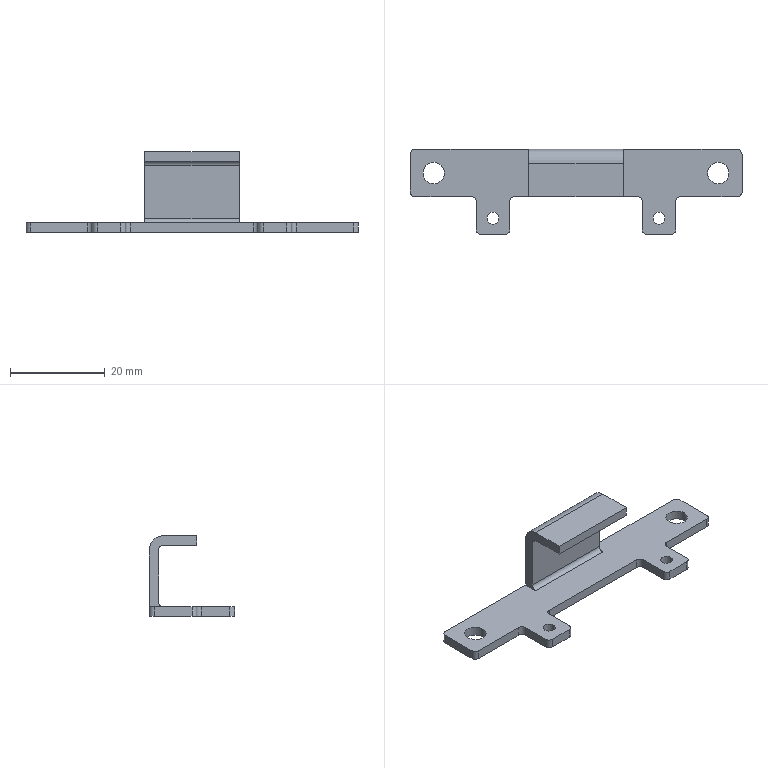Part | SolidWorks | features Fillet 4, ICE 4, 3DProfileFeature 1, Extrusion 1, HoleWzd 1 | 1 solid | 43 faces | box 70 x 18 x 17 mm | volume 2429 mm3 | cylinder 23 | plane 20 | commonest cylinder face diameters 2 x14 2.5 x4 4.5 x4 6 x1
STEP:
#1=CARTESIAN_POINT('',(-18.75,-9.5,0.));
#2=VERTEX_POINT('',#1);
#3=CARTESIAN_POINT('',(-16.25,-9.5,0.));
#4=VERTEX_POINT('',#3);
#5=CARTESIAN_POINT('',(-17.5,-9.5,0.));
#6=DIRECTION('',(0.,0.,1.));
#7=DIRECTION('',(1.,0.,0.));
#8=AXIS2_PLACEMENT_3D('',#5,#6,#7);
#9=CIRCLE('',#8,1.25);
#10=EDGE_CURVE('',#2,#4,#9,.T.);
#11=ORIENTED_EDGE('',*,*,#10,.F.);
#12=CARTESIAN_POINT('',(-18.75,-9.5,2.));
#13=VERTEX_POINT('',#12);
#14=CARTESIAN_POINT('',(-18.75,-9.5,2.));
#15=DIRECTION('',(0.,0.,1.));
#16=VECTOR('',#15,1000.);
#17=LINE('',#14,#16);
#18=EDGE_CURVE('',#2,#13,#17,.T.);
#19=ORIENTED_EDGE('',*,*,#18,.T.);
#20=CARTESIAN_POINT('',(-16.25,-9.5,2.));
#21=VERTEX_POINT('',#20);
#22=CARTESIAN_POINT('',(-17.5,-9.5,2.));
#23=DIRECTION('',(0.,0.,1.));
#24=DIRECTION('',(1.,0.,0.));
#25=AXIS2_PLACEMENT_3D('',#22,#23,#24);
#26=CIRCLE('',#25,1.25);
#27=EDGE_CURVE('',#13,#21,#26,.T.);
#28=ORIENTED_EDGE('',*,*,#27,.T.);
#29=CARTESIAN_POINT('',(-16.25,-9.5,2.));
#30=DIRECTION('',(0.,0.,1.));
#31=VECTOR('',#30,1000.);
#32=LINE('',#29,#31);
#33=EDGE_CURVE('',#4,#21,#32,.T.);
#34=ORIENTED_EDGE('',*,*,#33,.F.);
#35=EDGE_LOOP('',(#11,#19,#28,#34));
#36=FACE_OUTER_BOUND('',#35,.T.);
#37=CARTESIAN_POINT('',(-17.5,-9.5,2.));
#38=DIRECTION('',(0.,0.,1.));
#39=DIRECTION('',(1.,0.,0.));
#40=AXIS2_PLACEMENT_3D('',#37,#38,#39);
#41=CYLINDRICAL_SURFACE('',#40,1.25);
#42=ADVANCED_FACE('',(#36),#41,.F.);
#43=CARTESIAN_POINT('',(16.25,-9.5,0.));
#44=VERTEX_POINT('',#43);
#45=CARTESIAN_POINT('',(18.75,-9.5,0.));
#46=VERTEX_POINT('',#45);
#47=CARTESIAN_POINT('',(17.5,-9.5,0.));
#48=DIRECTION('',(0.,0.,1.));
#49=DIRECTION('',(1.,0.,0.));
#50=AXIS2_PLACEMENT_3D('',#47,#48,#49);
#51=CIRCLE('',#50,1.25);
#52=EDGE_CURVE('',#44,#46,#51,.T.);
#53=ORIENTED_EDGE('',*,*,#52,.F.);
#54=CARTESIAN_POINT('',(16.25,-9.5,2.));
#55=VERTEX_POINT('',#54);
#56=CARTESIAN_POINT('',(16.25,-9.5,2.));
#57=DIRECTION('',(0.,0.,1.));
#58=VECTOR('',#57,1000.);
#59=LINE('',#56,#58);
#60=EDGE_CURVE('',#44,#55,#59,.T.);
#61=ORIENTED_EDGE('',*,*,#60,.T.);
#62=CARTESIAN_POINT('',(18.75,-9.5,2.));
#63=VERTEX_POINT('',#62);
#64=CARTESIAN_POINT('',(17.5,-9.5,2.));
#65=DIRECTION('',(0.,0.,1.));
#66=DIRECTION('',(1.,0.,0.));
#67=AXIS2_PLACEMENT_3D('',#64,#65,#66);
#68=CIRCLE('',#67,1.25);
#69=EDGE_CURVE('',#55,#63,#68,.T.);
#70=ORIENTED_EDGE('',*,*,#69,.T.);
#71=CARTESIAN_POINT('',(18.75,-9.5,2.));
#72=DIRECTION('',(0.,0.,1.));
#73=VECTOR('',#72,1000.);
#74=LINE('',#71,#73);
#75=EDGE_CURVE('',#46,#63,#74,.T.);
#76=ORIENTED_EDGE('',*,*,#75,.F.);
#77=EDGE_LOOP('',(#53,#61,#70,#76));
#78=FACE_OUTER_BOUND('',#77,.T.);
#79=CARTESIAN_POINT('',(17.5,-9.5,2.));
#80=DIRECTION('',(0.,0.,1.));
#81=DIRECTION('',(1.,0.,0.));
#82=AXIS2_PLACEMENT_3D('',#79,#80,#81);
#83=CYLINDRICAL_SURFACE('',#82,1.25);
#84=ADVANCED_FACE('',(#78),#83,.F.);
#85=CARTESIAN_POINT('',(-32.25,0.,0.));
#86=VERTEX_POINT('',#85);
#87=CARTESIAN_POINT('',(-27.75,0.,0.));
#88=VERTEX_POINT('',#87);
#89=CARTESIAN_POINT('',(-30.,0.,0.));
#90=DIRECTION('',(0.,0.,1.));
#91=DIRECTION('',(1.,0.,0.));
#92=AXIS2_PLACEMENT_3D('',#89,#90,#91);
#93=CIRCLE('',#92,2.25);
#94=EDGE_CURVE('',#86,#88,#93,.T.);
#95=ORIENTED_EDGE('',*,*,#94,.F.);
#96=CARTESIAN_POINT('',(-32.25,0.,2.));
#97=VERTEX_POINT('',#96);
#98=CARTESIAN_POINT('',(-32.25,0.,-6.));
#99=DIRECTION('',(0.,0.,1.));
#100=VECTOR('',#99,1000.);
#101=LINE('',#98,#100);
#102=EDGE_CURVE('',#86,#97,#101,.T.);
#103=ORIENTED_EDGE('',*,*,#102,.T.);
#104=CARTESIAN_POINT('',(-27.75,0.,2.));
#105=VERTEX_POINT('',#104);
#106=CARTESIAN_POINT('',(-30.,0.,2.));
#107=DIRECTION('',(0.,0.,1.));
#108=DIRECTION('',(1.,0.,0.));
#109=AXIS2_PLACEMENT_3D('',#106,#107,#108);
#110=CIRCLE('',#109,2.25);
#111=EDGE_CURVE('',#97,#105,#110,.T.);
#112=ORIENTED_EDGE('',*,*,#111,.T.);
#113=CARTESIAN_POINT('',(-27.75,0.,-6.));
#114=DIRECTION('',(0.,0.,1.));
#115=VECTOR('',#114,1000.);
#116=LINE('',#113,#115);
#117=EDGE_CURVE('',#88,#105,#116,.T.);
#118=ORIENTED_EDGE('',*,*,#117,.F.);
#119=EDGE_LOOP('',(#95,#103,#112,#118));
#120=FACE_OUTER_BOUND('',#119,.T.);
#121=CARTESIAN_POINT('',(-30.,0.,-6.));
#122=DIRECTION('',(0.,0.,1.));
#123=DIRECTION('',(1.,0.,0.));
#124=AXIS2_PLACEMENT_3D('',#121,#122,#123);
#125=CYLINDRICAL_SURFACE('',#124,2.25);
#126=ADVANCED_FACE('',(#120),#125,.F.);
#127=CARTESIAN_POINT('',(27.75,0.,0.));
#128=VERTEX_POINT('',#127);
#129=CARTESIAN_POINT('',(32.25,0.,0.));
#130=VERTEX_POINT('',#129);
#131=CARTESIAN_POINT('',(30.,0.,0.));
#132=DIRECTION('',(0.,0.,1.));
#133=DIRECTION('',(1.,0.,0.));
#134=AXIS2_PLACEMENT_3D('',#131,#132,#133);
#135=CIRCLE('',#134,2.25);
#136=EDGE_CURVE('',#128,#130,#135,.T.);
#137=ORIENTED_EDGE('',*,*,#136,.F.);
#138=CARTESIAN_POINT('',(27.75,0.,2.));
#139=VERTEX_POINT('',#138);
#140=CARTESIAN_POINT('',(27.75,0.,-6.));
#141=DIRECTION('',(0.,0.,1.));
#142=VECTOR('',#141,1000.);
#143=LINE('',#140,#142);
#144=EDGE_CURVE('',#128,#139,#143,.T.);
#145=ORIENTED_EDGE('',*,*,#144,.T.);
#146=CARTESIAN_POINT('',(32.25,0.,2.));
#147=VERTEX_POINT('',#146);
#148=CARTESIAN_POINT('',(30.,0.,2.));
#149=DIRECTION('',(0.,0.,1.));
#150=DIRECTION('',(1.,0.,0.));
#151=AXIS2_PLACEMENT_3D('',#148,#149,#150);
#152=CIRCLE('',#151,2.25);
#153=EDGE_CURVE('',#139,#147,#152,.T.);
#154=ORIENTED_EDGE('',*,*,#153,.T.);
#155=CARTESIAN_POINT('',(32.25,0.,-6.));
#156=DIRECTION('',(0.,0.,1.));
#157=VECTOR('',#156,1000.);
#158=LINE('',#155,#157);
#159=EDGE_CURVE('',#130,#147,#158,.T.);
#160=ORIENTED_EDGE('',*,*,#159,.F.);
#161=EDGE_LOOP('',(#137,#145,#154,#160));
#162=FACE_OUTER_BOUND('',#161,.T.);
#163=CARTESIAN_POINT('',(30.,0.,-6.));
#164=DIRECTION('',(0.,0.,1.));
#165=DIRECTION('',(1.,0.,0.));
#166=AXIS2_PLACEMENT_3D('',#163,#164,#165);
#167=CYLINDRICAL_SURFACE('',#166,2.25);
#168=ADVANCED_FACE('',(#162),#167,.F.);
#169=CARTESIAN_POINT('',(-13.,-5.,2.));
#170=VERTEX_POINT('',#169);
#171=CARTESIAN_POINT('',(13.,-5.,2.));
#172=VERTEX_POINT('',#171);
#173=CARTESIAN_POINT('',(-35.,-5.,2.));
#174=DIRECTION('',(1.,0.,0.));
#175=VECTOR('',#174,1000.);
#176=LINE('',#173,#175);
#177=EDGE_CURVE('',#170,#172,#176,.T.);
#178=ORIENTED_EDGE('',*,*,#177,.F.);
#179=CARTESIAN_POINT('',(-13.,-5.,0.));
#180=VERTEX_POINT('',#179);
#181=CARTESIAN_POINT('',(-13.,-5.,0.));
#182=DIRECTION('',(0.,0.,-1.));
#183=VECTOR('',#182,1000.);
#184=LINE('',#181,#183);
#185=EDGE_CURVE('',#170,#180,#184,.T.);
#186=ORIENTED_EDGE('',*,*,#185,.T.);
#187=CARTESIAN_POINT('',(13.,-5.,0.));
#188=VERTEX_POINT('',#187);
#189=CARTESIAN_POINT('',(-35.,-5.,0.));
#190=DIRECTION('',(1.,0.,0.));
#191=VECTOR('',#190,1000.);
#192=LINE('',#189,#191);
#193=EDGE_CURVE('',#180,#188,#192,.T.);
#194=ORIENTED_EDGE('',*,*,#193,.T.);
#195=CARTESIAN_POINT('',(13.,-5.,2.));
#196=DIRECTION('',(0.,0.,1.));
#197=VECTOR('',#196,1000.);
#198=LINE('',#195,#197);
#199=EDGE_CURVE('',#188,#172,#198,.T.);
#200=ORIENTED_EDGE('',*,*,#199,.T.);
#201=EDGE_LOOP('',(#178,#186,#194,#200));
#202=FACE_OUTER_BOUND('',#201,.T.);
#203=CARTESIAN_POINT('',(-35.,-5.,2.));
#204=DIRECTION('',(0.,1.,0.));
#205=DIRECTION('',(0.,0.,1.));
#206=AXIS2_PLACEMENT_3D('',#203,#204,#205);
#207=PLANE('',#206);
#208=ADVANCED_FACE('',(#202),#207,.F.);
#209=CARTESIAN_POINT('',(22.,-5.,2.));
#210=VERTEX_POINT('',#209);
#211=CARTESIAN_POINT('',(34.,-5.,2.));
#212=VERTEX_POINT('',#211);
#213=CARTESIAN_POINT('',(-35.,-5.,2.));
#214=DIRECTION('',(1.,0.,0.));
#215=VECTOR('',#214,1000.);
#216=LINE('',#213,#215);
#217=EDGE_CURVE('',#210,#212,#216,.T.);
#218=ORIENTED_EDGE('',*,*,#217,.F.);
#219=CARTESIAN_POINT('',(22.,-5.,0.));
#220=VERTEX_POINT('',#219);
#221=CARTESIAN_POINT('',(22.,-5.,0.));
#222=DIRECTION('',(0.,0.,-1.));
#223=VECTOR('',#222,1000.);
#224=LINE('',#221,#223);
#225=EDGE_CURVE('',#210,#220,#224,.T.);
#226=ORIENTED_EDGE('',*,*,#225,.T.);
#227=CARTESIAN_POINT('',(34.,-5.,0.));
#228=VERTEX_POINT('',#227);
#229=CARTESIAN_POINT('',(-35.,-5.,0.));
#230=DIRECTION('',(1.,0.,0.));
#231=VECTOR('',#230,1000.);
#232=LINE('',#229,#231);
#233=EDGE_CURVE('',#220,#228,#232,.T.);
#234=ORIENTED_EDGE('',*,*,#233,.T.);
#235=CARTESIAN_POINT('',(34.,-5.,2.));
#236=DIRECTION('',(0.,0.,1.));
#237=VECTOR('',#236,1000.);
#238=LINE('',#235,#237);
#239=EDGE_CURVE('',#228,#212,#238,.T.);
#240=ORIENTED_EDGE('',*,*,#239,.T.);
#241=EDGE_LOOP('',(#218,#226,#234,#240));
#242=FACE_OUTER_BOUND('',#241,.T.);
#243=CARTESIAN_POINT('',(-35.,-5.,2.));
#244=DIRECTION('',(0.,1.,0.));
#245=DIRECTION('',(0.,0.,1.));
#246=AXIS2_PLACEMENT_3D('',#243,#244,#245);
#247=PLANE('',#246);
#248=ADVANCED_FACE('',(#242),#247,.F.);
#249=CARTESIAN_POINT('',(-34.,-5.,0.));
#250=VERTEX_POINT('',#249);
#251=CARTESIAN_POINT('',(-22.,-5.,0.));
#252=VERTEX_POINT('',#251);
#253=CARTESIAN_POINT('',(-35.,-5.,0.));
#254=DIRECTION('',(1.,0.,0.));
#255=VECTOR('',#254,1000.);
#256=LINE('',#253,#255);
#257=EDGE_CURVE('',#250,#252,#256,.T.);
#258=ORIENTED_EDGE('',*,*,#257,.T.);
#259=CARTESIAN_POINT('',(-22.,-5.,2.));
#260=VERTEX_POINT('',#259);
#261=CARTESIAN_POINT('',(-22.,-5.,2.));
#262=DIRECTION('',(0.,0.,1.));
#263=VECTOR('',#262,1000.);
#264=LINE('',#261,#263);
#265=EDGE_CURVE('',#252,#260,#264,.T.);
#266=ORIENTED_EDGE('',*,*,#265,.T.);
#267=CARTESIAN_POINT('',(-34.,-5.,2.));
#268=VERTEX_POINT('',#267);
#269=CARTESIAN_POINT('',(-35.,-5.,2.));
#270=DIRECTION('',(1.,0.,0.));
#271=VECTOR('',#270,1000.);
#272=LINE('',#269,#271);
#273=EDGE_CURVE('',#268,#260,#272,.T.);
#274=ORIENTED_EDGE('',*,*,#273,.F.);
#275=CARTESIAN_POINT('',(-34.,-5.,2.));
#276=DIRECTION('',(0.,0.,-1.));
#277=VECTOR('',#276,1000.);
#278=LINE('',#275,#277);
#279=EDGE_CURVE('',#268,#250,#278,.T.);
#280=ORIENTED_EDGE('',*,*,#279,.T.);
#281=EDGE_LOOP('',(#258,#266,#274,#280));
#282=FACE_OUTER_BOUND('',#281,.T.);
#283=CARTESIAN_POINT('',(-35.,-5.,2.));
#284=DIRECTION('',(0.,1.,0.));
#285=DIRECTION('',(0.,0.,1.));
#286=AXIS2_PLACEMENT_3D('',#283,#284,#285);
#287=PLANE('',#286);
#288=ADVANCED_FACE('',(#282),#287,.F.);
#289=CARTESIAN_POINT('',(-10.,3.,14.));
#290=VERTEX_POINT('',#289);
#291=CARTESIAN_POINT('',(-10.,3.,3.));
#292=VERTEX_POINT('',#291);
#293=CARTESIAN_POINT('',(-10.,3.,17.));
#294=DIRECTION('',(0.,0.,-1.));
#295=VECTOR('',#294,1000.);
#296=LINE('',#293,#295);
#297=EDGE_CURVE('',#290,#292,#296,.T.);
#298=ORIENTED_EDGE('',*,*,#297,.T.);
#299=CARTESIAN_POINT('',(10.,3.,3.));
#300=VERTEX_POINT('',#299);
#301=CARTESIAN_POINT('',(-10.,3.,3.));
#302=DIRECTION('',(1.,0.,0.));
#303=VECTOR('',#302,1000.);
#304=LINE('',#301,#303);
#305=EDGE_CURVE('',#292,#300,#304,.T.);
#306=ORIENTED_EDGE('',*,*,#305,.T.);
#307=CARTESIAN_POINT('',(10.,3.,14.));
#308=VERTEX_POINT('',#307);
#309=CARTESIAN_POINT('',(10.,3.,17.));
#310=DIRECTION('',(0.,0.,-1.));
#311=VECTOR('',#310,1000.);
#312=LINE('',#309,#311);
#313=EDGE_CURVE('',#308,#300,#312,.T.);
#314=ORIENTED_EDGE('',*,*,#313,.F.);
#315=CARTESIAN_POINT('',(-10.,3.,14.));
#316=DIRECTION('',(-1.,0.,0.));
#317=VECTOR('',#316,1000.);
#318=LINE('',#315,#317);
#319=EDGE_CURVE('',#308,#290,#318,.T.);
#320=ORIENTED_EDGE('',*,*,#319,.T.);
#321=EDGE_LOOP('',(#298,#306,#314,#320));
#322=FACE_OUTER_BOUND('',#321,.T.);
#323=CARTESIAN_POINT('',(-10.,3.,17.));
#324=DIRECTION('',(0.,1.,0.));
#325=DIRECTION('',(0.,0.,1.));
#326=AXIS2_PLACEMENT_3D('',#323,#324,#325);
#327=PLANE('',#326);
#328=ADVANCED_FACE('',(#322),#327,.F.);
#329=CARTESIAN_POINT('',(35.,-4.,0.));
#330=VERTEX_POINT('',#329);
#331=CARTESIAN_POINT('',(35.,4.,0.));
#332=VERTEX_POINT('',#331);
#333=CARTESIAN_POINT('',(35.,5.,0.));
#334=DIRECTION('',(0.,1.,0.));
#335=VECTOR('',#334,1000.);
#336=LINE('',#333,#335);
#337=EDGE_CURVE('',#330,#332,#336,.T.);
#338=ORIENTED_EDGE('',*,*,#337,.T.);
#339=CARTESIAN_POINT('',(35.,4.,2.));
#340=VERTEX_POINT('',#339);
#341=CARTESIAN_POINT('',(35.,4.,2.));
#342=DIRECTION('',(0.,0.,1.));
#343=VECTOR('',#342,1000.);
#344=LINE('',#341,#343);
#345=EDGE_CURVE('',#332,#340,#344,.T.);
#346=ORIENTED_EDGE('',*,*,#345,.T.);
#347=CARTESIAN_POINT('',(35.,-4.,2.));
#348=VERTEX_POINT('',#347);
#349=CARTESIAN_POINT('',(35.,5.,2.));
#350=DIRECTION('',(0.,1.,0.));
#351=VECTOR('',#350,1000.);
#352=LINE('',#349,#351);
#353=EDGE_CURVE('',#348,#340,#352,.T.);
#354=ORIENTED_EDGE('',*,*,#353,.F.);
#355=CARTESIAN_POINT('',(35.,-4.,2.));
#356=DIRECTION('',(0.,0.,-1.));
#357=VECTOR('',#356,1000.);
#358=LINE('',#355,#357);
#359=EDGE_CURVE('',#348,#330,#358,.T.);
#360=ORIENTED_EDGE('',*,*,#359,.T.);
#361=EDGE_LOOP('',(#338,#346,#354,#360));
#362=FACE_OUTER_BOUND('',#361,.T.);
#363=CARTESIAN_POINT('',(35.,5.,2.));
#364=DIRECTION('',(-1.,0.,0.));
#365=DIRECTION('',(0.,0.,1.));
#366=AXIS2_PLACEMENT_3D('',#363,#364,#365);
#367=PLANE('',#366);
#368=ADVANCED_FACE('',(#362),#367,.F.);
#369=CARTESIAN_POINT('',(34.,5.,2.));
#370=VERTEX_POINT('',#369);
#371=CARTESIAN_POINT('',(10.,5.,2.));
#372=VERTEX_POINT('',#371);
#373=CARTESIAN_POINT('',(-35.,5.,2.));
#374=DIRECTION('',(-1.,0.,0.));
#375=VECTOR('',#374,1000.);
#376=LINE('',#373,#375);
#377=EDGE_CURVE('',#370,#372,#376,.T.);
#378=ORIENTED_EDGE('',*,*,#377,.F.);
#379=CARTESIAN_POINT('',(34.,5.,0.));
#380=VERTEX_POINT('',#379);
#381=CARTESIAN_POINT('',(34.,5.,2.));
#382=DIRECTION('',(0.,0.,-1.));
#383=VECTOR('',#382,1000.);
#384=LINE('',#381,#383);
#385=EDGE_CURVE('',#370,#380,#384,.T.);
#386=ORIENTED_EDGE('',*,*,#385,.T.);
#387=CARTESIAN_POINT('',(-34.,5.,0.));
#388=VERTEX_POINT('',#387);
#389=CARTESIAN_POINT('',(-35.,5.,0.));
#390=DIRECTION('',(-1.,0.,0.));
#391=VECTOR('',#390,1000.);
#392=LINE('',#389,#391);
#393=EDGE_CURVE('',#380,#388,#392,.T.);
#394=ORIENTED_EDGE('',*,*,#393,.T.);
#395=CARTESIAN_POINT('',(-34.,5.,2.));
#396=VERTEX_POINT('',#395);
#397=CARTESIAN_POINT('',(-34.,5.,2.));
#398=DIRECTION('',(0.,0.,1.));
#399=VECTOR('',#398,1000.);
#400=LINE('',#397,#399);
#401=EDGE_CURVE('',#388,#396,#400,.T.);
#402=ORIENTED_EDGE('',*,*,#401,.T.);
#403=CARTESIAN_POINT('',(-10.,5.,2.));
#404=VERTEX_POINT('',#403);
#405=CARTESIAN_POINT('',(-35.,5.,2.));
#406=DIRECTION('',(-1.,0.,0.));
#407=VECTOR('',#406,1000.);
#408=LINE('',#405,#407);
#409=EDGE_CURVE('',#404,#396,#408,.T.);
#410=ORIENTED_EDGE('',*,*,#409,.F.);
#411=CARTESIAN_POINT('',(-10.,5.,14.));
#412=VERTEX_POINT('',#411);
#413=CARTESIAN_POINT('',(-10.,5.,17.));
#414=DIRECTION('',(0.,0.,-1.));
#415=VECTOR('',#414,1000.);
#416=LINE('',#413,#415);
#417=EDGE_CURVE('',#412,#404,#416,.T.);
#418=ORIENTED_EDGE('',*,*,#417,.F.);
#419=CARTESIAN_POINT('',(10.,5.,14.));
#420=VERTEX_POINT('',#419);
#421=CARTESIAN_POINT('',(-35.,5.,14.));
#422=DIRECTION('',(1.,0.,0.));
#423=VECTOR('',#422,1000.);
#424=LINE('',#421,#423);
#425=EDGE_CURVE('',#412,#420,#424,.T.);
#426=ORIENTED_EDGE('',*,*,#425,.T.);
#427=CARTESIAN_POINT('',(10.,5.,17.));
#428=DIRECTION('',(0.,0.,-1.));
#429=VECTOR('',#428,1000.);
#430=LINE('',#427,#429);
#431=EDGE_CURVE('',#420,#372,#430,.T.);
#432=ORIENTED_EDGE('',*,*,#431,.T.);
#433=EDGE_LOOP('',(#378,#386,#394,#402,#410,#418,#426,#432));
#434=FACE_OUTER_BOUND('',#433,.T.);
#435=CARTESIAN_POINT('',(-35.,5.,2.));
#436=DIRECTION('',(0.,-1.,0.));
#437=DIRECTION('',(0.,0.,-1.));
#438=AXIS2_PLACEMENT_3D('',#435,#436,#437);
#439=PLANE('',#438);
#440=ADVANCED_FACE('',(#434),#439,.F.);
#441=CARTESIAN_POINT('',(-35.,4.,0.));
#442=VERTEX_POINT('',#441);
#443=CARTESIAN_POINT('',(-35.,-4.,0.));
#444=VERTEX_POINT('',#443);
#445=CARTESIAN_POINT('',(-35.,5.,0.));
#446=DIRECTION('',(0.,-1.,0.));
#447=VECTOR('',#446,1000.);
#448=LINE('',#445,#447);
#449=EDGE_CURVE('',#442,#444,#448,.T.);
#450=ORIENTED_EDGE('',*,*,#449,.T.);
#451=CARTESIAN_POINT('',(-35.,-4.,2.));
#452=VERTEX_POINT('',#451);
#453=CARTESIAN_POINT('',(-35.,-4.,2.));
#454=DIRECTION('',(0.,0.,1.));
#455=VECTOR('',#454,1000.);
#456=LINE('',#453,#455);
#457=EDGE_CURVE('',#444,#452,#456,.T.);
#458=ORIENTED_EDGE('',*,*,#457,.T.);
#459=CARTESIAN_POINT('',(-35.,4.,2.));
#460=VERTEX_POINT('',#459);
#461=CARTESIAN_POINT('',(-35.,5.,2.));
#462=DIRECTION('',(0.,-1.,0.));
#463=VECTOR('',#462,1000.);
#464=LINE('',#461,#463);
#465=EDGE_CURVE('',#460,#452,#464,.T.);
#466=ORIENTED_EDGE('',*,*,#465,.F.);
#467=CARTESIAN_POINT('',(-35.,4.,2.));
#468=DIRECTION('',(0.,0.,-1.));
#469=VECTOR('',#468,1000.);
#470=LINE('',#467,#469);
#471=EDGE_CURVE('',#460,#442,#470,.T.);
#472=ORIENTED_EDGE('',*,*,#471,.T.);
#473=EDGE_LOOP('',(#450,#458,#466,#472));
#474=FACE_OUTER_BOUND('',#473,.T.);
#475=CARTESIAN_POINT('',(-35.,5.,2.));
#476=DIRECTION('',(1.,0.,0.));
#477=DIRECTION('',(0.,0.,-1.));
#478=AXIS2_PLACEMENT_3D('',#475,#476,#477);
#479=PLANE('',#478);
#480=ADVANCED_FACE('',(#474),#479,.F.);
#481=CARTESIAN_POINT('',(-17.5,-9.5,2.));
#482=DIRECTION('',(0.,0.,1.));
#483=DIRECTION('',(1.,0.,0.));
#484=AXIS2_PLACEMENT_3D('',#481,#482,#483);
#485=CIRCLE('',#484,1.25);
#486=EDGE_CURVE('',#21,#13,#485,.T.);
#487=ORIENTED_EDGE('',*,*,#486,.F.);
#488=ORIENTED_EDGE('',*,*,#27,.F.);
#489=EDGE_LOOP('',(#487,#488));
#490=FACE_BOUND('',#489,.T.);
#491=CARTESIAN_POINT('',(17.5,-9.5,2.));
#492=DIRECTION('',(0.,0.,1.));
#493=DIRECTION('',(1.,0.,0.));
#494=AXIS2_PLACEMENT_3D('',#491,#492,#493);
#495=CIRCLE('',#494,1.25);
#496=EDGE_CURVE('',#63,#55,#495,.T.);
#497=ORIENTED_EDGE('',*,*,#496,.F.);
#498=ORIENTED_EDGE('',*,*,#69,.F.);
#499=EDGE_LOOP('',(#497,#498));
#500=FACE_BOUND('',#499,.T.);
#501=CARTESIAN_POINT('',(-30.,0.,2.));
#502=DIRECTION('',(0.,0.,1.));
#503=DIRECTION('',(1.,0.,0.));
#504=AXIS2_PLACEMENT_3D('',#501,#502,#503);
#505=CIRCLE('',#504,2.25);
#506=EDGE_CURVE('',#105,#97,#505,.T.);
#507=ORIENTED_EDGE('',*,*,#506,.F.);
#508=ORIENTED_EDGE('',*,*,#111,.F.);
#509=EDGE_LOOP('',(#507,#508));
#510=FACE_BOUND('',#509,.T.);
#511=CARTESIAN_POINT('',(30.,0.,2.));
#512=DIRECTION('',(0.,0.,1.));
#513=DIRECTION('',(1.,0.,0.));
#514=AXIS2_PLACEMENT_3D('',#511,#512,#513);
#515=CIRCLE('',#514,2.25);
#516=EDGE_CURVE('',#147,#139,#515,.T.);
#517=ORIENTED_EDGE('',*,*,#516,.F.);
#518=ORIENTED_EDGE('',*,*,#153,.F.);
#519=EDGE_LOOP('',(#517,#518));
#520=FACE_BOUND('',#519,.T.);
#521=CARTESIAN_POINT('',(-21.,-12.,2.));
#522=VERTEX_POINT('',#521);
#523=CARTESIAN_POINT('',(-21.,-6.,2.));
#524=VERTEX_POINT('',#523);
#525=CARTESIAN_POINT('',(-21.,-13.,2.));
#526=DIRECTION('',(0.,1.,0.));
#527=VECTOR('',#526,1000.);
#528=LINE('',#525,#527);
#529=EDGE_CURVE('',#522,#524,#528,.T.);
#530=ORIENTED_EDGE('',*,*,#529,.F.);
#531=CARTESIAN_POINT('',(-20.,-13.,2.));
#532=VERTEX_POINT('',#531);
#533=CARTESIAN_POINT('',(-20.,-12.,2.));
#534=DIRECTION('',(0.,0.,1.));
#535=DIRECTION('',(1.,0.,0.));
#536=AXIS2_PLACEMENT_3D('',#533,#534,#535);
#537=CIRCLE('',#536,1.);
#538=EDGE_CURVE('',#522,#532,#537,.T.);
#539=ORIENTED_EDGE('',*,*,#538,.T.);
#540=CARTESIAN_POINT('',(-15.,-13.,2.));
#541=VERTEX_POINT('',#540);
#542=CARTESIAN_POINT('',(-14.,-13.,2.));
#543=DIRECTION('',(-1.,0.,0.));
#544=VECTOR('',#543,1000.);
#545=LINE('',#542,#544);
#546=EDGE_CURVE('',#541,#532,#545,.T.);
#547=ORIENTED_EDGE('',*,*,#546,.F.);
#548=CARTESIAN_POINT('',(-14.,-12.,2.));
#549=VERTEX_POINT('',#548);
#550=CARTESIAN_POINT('',(-15.,-12.,2.));
#551=DIRECTION('',(0.,0.,1.));
#552=DIRECTION('',(1.,0.,0.));
#553=AXIS2_PLACEMENT_3D('',#550,#551,#552);
#554=CIRCLE('',#553,1.);
#555=EDGE_CURVE('',#541,#549,#554,.T.);
#556=ORIENTED_EDGE('',*,*,#555,.T.);
#557=CARTESIAN_POINT('',(-14.,-6.,2.));
#558=VERTEX_POINT('',#557);
#559=CARTESIAN_POINT('',(-14.,-13.,2.));
#560=DIRECTION('',(0.,1.,0.));
#561=VECTOR('',#560,1000.);
#562=LINE('',#559,#561);
#563=EDGE_CURVE('',#549,#558,#562,.T.);
#564=ORIENTED_EDGE('',*,*,#563,.T.);
#565=CARTESIAN_POINT('',(-13.,-6.,2.));
#566=DIRECTION('',(0.,0.,-1.));
#567=DIRECTION('',(1.,0.,0.));
#568=AXIS2_PLACEMENT_3D('',#565,#566,#567);
#569=CIRCLE('',#568,1.);
#570=EDGE_CURVE('',#558,#170,#569,.T.);
#571=ORIENTED_EDGE('',*,*,#570,.T.);
#572=ORIENTED_EDGE('',*,*,#177,.T.);
#573=CARTESIAN_POINT('',(14.,-6.,2.));
#574=VERTEX_POINT('',#573);
#575=CARTESIAN_POINT('',(13.,-6.,2.));
#576=DIRECTION('',(0.,0.,-1.));
#577=DIRECTION('',(1.,0.,0.));
#578=AXIS2_PLACEMENT_3D('',#575,#576,#577);
#579=CIRCLE('',#578,1.);
#580=EDGE_CURVE('',#172,#574,#579,.T.);
#581=ORIENTED_EDGE('',*,*,#580,.T.);
#582=CARTESIAN_POINT('',(14.,-12.,2.));
#583=VERTEX_POINT('',#582);
#584=CARTESIAN_POINT('',(14.,-13.,2.));
#585=DIRECTION('',(0.,1.,0.));
#586=VECTOR('',#585,1000.);
#587=LINE('',#584,#586);
#588=EDGE_CURVE('',#583,#574,#587,.T.);
#589=ORIENTED_EDGE('',*,*,#588,.F.);
#590=CARTESIAN_POINT('',(15.,-13.,2.));
#591=VERTEX_POINT('',#590);
#592=CARTESIAN_POINT('',(15.,-12.,2.));
#593=DIRECTION('',(0.,0.,1.));
#594=DIRECTION('',(1.,0.,0.));
#595=AXIS2_PLACEMENT_3D('',#592,#593,#594);
#596=CIRCLE('',#595,1.);
#597=EDGE_CURVE('',#583,#591,#596,.T.);
#598=ORIENTED_EDGE('',*,*,#597,.T.);
#599=CARTESIAN_POINT('',(20.,-13.,2.));
#600=VERTEX_POINT('',#599);
#601=CARTESIAN_POINT('',(21.,-13.,2.));
#602=DIRECTION('',(-1.,0.,0.));
#603=VECTOR('',#602,1000.);
#604=LINE('',#601,#603);
#605=EDGE_CURVE('',#600,#591,#604,.T.);
#606=ORIENTED_EDGE('',*,*,#605,.F.);
#607=CARTESIAN_POINT('',(21.,-12.,2.));
#608=VERTEX_POINT('',#607);
#609=CARTESIAN_POINT('',(20.,-12.,2.));
#610=DIRECTION('',(0.,0.,1.));
#611=DIRECTION('',(1.,0.,0.));
#612=AXIS2_PLACEMENT_3D('',#609,#610,#611);
#613=CIRCLE('',#612,1.);
#614=EDGE_CURVE('',#600,#608,#613,.T.);
#615=ORIENTED_EDGE('',*,*,#614,.T.);
#616=CARTESIAN_POINT('',(21.,-6.,2.));
#617=VERTEX_POINT('',#616);
#618=CARTESIAN_POINT('',(21.,-13.,2.));
#619=DIRECTION('',(0.,1.,0.));
#620=VECTOR('',#619,1000.);
#621=LINE('',#618,#620);
#622=EDGE_CURVE('',#608,#617,#621,.T.);
#623=ORIENTED_EDGE('',*,*,#622,.T.);
#624=CARTESIAN_POINT('',(22.,-6.,2.));
#625=DIRECTION('',(0.,0.,-1.));
#626=DIRECTION('',(1.,0.,0.));
#627=AXIS2_PLACEMENT_3D('',#624,#625,#626);
#628=CIRCLE('',#627,1.);
#629=EDGE_CURVE('',#617,#210,#628,.T.);
#630=ORIENTED_EDGE('',*,*,#629,.T.);
#631=ORIENTED_EDGE('',*,*,#217,.T.);
#632=CARTESIAN_POINT('',(34.,-4.,2.));
#633=DIRECTION('',(0.,0.,1.));
#634=DIRECTION('',(1.,0.,0.));
#635=AXIS2_PLACEMENT_3D('',#632,#633,#634);
#636=CIRCLE('',#635,1.);
#637=EDGE_CURVE('',#212,#348,#636,.T.);
#638=ORIENTED_EDGE('',*,*,#637,.T.);
#639=ORIENTED_EDGE('',*,*,#353,.T.);
#640=CARTESIAN_POINT('',(34.,4.,2.));
#641=DIRECTION('',(0.,0.,1.));
#642=DIRECTION('',(1.,0.,0.));
#643=AXIS2_PLACEMENT_3D('',#640,#641,#642);
#644=CIRCLE('',#643,1.);
#645=EDGE_CURVE('',#340,#370,#644,.T.);
#646=ORIENTED_EDGE('',*,*,#645,.T.);
#647=ORIENTED_EDGE('',*,*,#377,.T.);
#648=CARTESIAN_POINT('',(10.,2.,2.));
#649=VERTEX_POINT('',#648);
#650=CARTESIAN_POINT('',(10.,3.,2.));
#651=DIRECTION('',(0.,1.,0.));
#652=VECTOR('',#651,1000.);
#653=LINE('',#650,#652);
#654=EDGE_CURVE('',#649,#372,#653,.T.);
#655=ORIENTED_EDGE('',*,*,#654,.F.);
#656=CARTESIAN_POINT('',(-10.,2.,2.));
#657=VERTEX_POINT('',#656);
#658=CARTESIAN_POINT('',(0.,2.,2.));
#659=DIRECTION('',(-1.,0.,0.));
#660=VECTOR('',#659,1000.);
#661=LINE('',#658,#660);
#662=EDGE_CURVE('',#649,#657,#661,.T.);
#663=ORIENTED_EDGE('',*,*,#662,.T.);
#664=CARTESIAN_POINT('',(-10.,3.,2.));
#665=DIRECTION('',(0.,-1.,0.));
#666=VECTOR('',#665,1000.);
#667=LINE('',#664,#666);
#668=EDGE_CURVE('',#404,#657,#667,.T.);
#669=ORIENTED_EDGE('',*,*,#668,.F.);
#670=ORIENTED_EDGE('',*,*,#409,.T.);
#671=CARTESIAN_POINT('',(-34.,4.,2.));
#672=DIRECTION('',(0.,0.,1.));
#673=DIRECTION('',(1.,0.,0.));
#674=AXIS2_PLACEMENT_3D('',#671,#672,#673);
#675=CIRCLE('',#674,1.);
#676=EDGE_CURVE('',#396,#460,#675,.T.);
#677=ORIENTED_EDGE('',*,*,#676,.T.);
#678=ORIENTED_EDGE('',*,*,#465,.T.);
#679=CARTESIAN_POINT('',(-34.,-4.,2.));
#680=DIRECTION('',(0.,0.,1.));
#681=DIRECTION('',(1.,0.,0.));
#682=AXIS2_PLACEMENT_3D('',#679,#680,#681);
#683=CIRCLE('',#682,1.);
#684=EDGE_CURVE('',#452,#268,#683,.T.);
#685=ORIENTED_EDGE('',*,*,#684,.T.);
#686=ORIENTED_EDGE('',*,*,#273,.T.);
#687=CARTESIAN_POINT('',(-22.,-6.,2.));
#688=DIRECTION('',(0.,0.,-1.));
#689=DIRECTION('',(1.,0.,0.));
#690=AXIS2_PLACEMENT_3D('',#687,#688,#689);
#691=CIRCLE('',#690,1.);
#692=EDGE_CURVE('',#260,#524,#691,.T.);
#693=ORIENTED_EDGE('',*,*,#692,.T.);
#694=EDGE_LOOP('',(#530,#539,#547,#556,#564,#571,#572,#581,#589,#598,#606,#615,#623,#630,#631,#638,#639,#646,#647,#655,#663,#669,#670,#677,#678,#685,#686,#693));
#695=FACE_OUTER_BOUND('',#694,.T.);
#696=CARTESIAN_POINT('',(0.,0.,2.));
#697=DIRECTION('',(0.,0.,1.));
#698=DIRECTION('',(1.,0.,0.));
#699=AXIS2_PLACEMENT_3D('',#696,#697,#698);
#700=PLANE('',#699);
#701=ADVANCED_FACE('',(#490,#500,#510,#520,#695),#700,.T.);
#702=CARTESIAN_POINT('',(-17.5,-9.5,0.));
#703=DIRECTION('',(0.,0.,1.));
#704=DIRECTION('',(1.,0.,0.));
#705=AXIS2_PLACEMENT_3D('',#702,#703,#704);
#706=CIRCLE('',#705,1.25);
#707=EDGE_CURVE('',#4,#2,#706,.T.);
#708=ORIENTED_EDGE('',*,*,#707,.T.);
#709=ORIENTED_EDGE('',*,*,#10,.T.);
#710=EDGE_LOOP('',(#708,#709));
#711=FACE_BOUND('',#710,.T.);
#712=CARTESIAN_POINT('',(17.5,-9.5,0.));
#713=DIRECTION('',(0.,0.,1.));
#714=DIRECTION('',(1.,0.,0.));
#715=AXIS2_PLACEMENT_3D('',#712,#713,#714);
#716=CIRCLE('',#715,1.25);
#717=EDGE_CURVE('',#46,#44,#716,.T.);
#718=ORIENTED_EDGE('',*,*,#717,.T.);
#719=ORIENTED_EDGE('',*,*,#52,.T.);
#720=EDGE_LOOP('',(#718,#719));
#721=FACE_BOUND('',#720,.T.);
#722=CARTESIAN_POINT('',(-30.,0.,0.));
#723=DIRECTION('',(0.,0.,1.));
#724=DIRECTION('',(1.,0.,0.));
#725=AXIS2_PLACEMENT_3D('',#722,#723,#724);
#726=CIRCLE('',#725,2.25);
#727=EDGE_CURVE('',#88,#86,#726,.T.);
#728=ORIENTED_EDGE('',*,*,#727,.T.);
#729=ORIENTED_EDGE('',*,*,#94,.T.);
#730=EDGE_LOOP('',(#728,#729));
#731=FACE_BOUND('',#730,.T.);
#732=CARTESIAN_POINT('',(30.,0.,0.));
#733=DIRECTION('',(0.,0.,1.));
#734=DIRECTION('',(1.,0.,0.));
#735=AXIS2_PLACEMENT_3D('',#732,#733,#734);
#736=CIRCLE('',#735,2.25);
#737=EDGE_CURVE('',#130,#128,#736,.T.);
#738=ORIENTED_EDGE('',*,*,#737,.T.);
#739=ORIENTED_EDGE('',*,*,#136,.T.);
#740=EDGE_LOOP('',(#738,#739));
#741=FACE_BOUND('',#740,.T.);
#742=CARTESIAN_POINT('',(-20.,-13.,0.));
#743=VERTEX_POINT('',#742);
#744=CARTESIAN_POINT('',(-15.,-13.,0.));
#745=VERTEX_POINT('',#744);
#746=CARTESIAN_POINT('',(-14.,-13.,0.));
#747=DIRECTION('',(1.,0.,0.));
#748=VECTOR('',#747,1000.);
#749=LINE('',#746,#748);
#750=EDGE_CURVE('',#743,#745,#749,.T.);
#751=ORIENTED_EDGE('',*,*,#750,.F.);
#752=CARTESIAN_POINT('',(-21.,-12.,0.));
#753=VERTEX_POINT('',#752);
#754=CARTESIAN_POINT('',(-20.,-12.,0.));
#755=DIRECTION('',(0.,0.,-1.));
#756=DIRECTION('',(1.,0.,0.));
#757=AXIS2_PLACEMENT_3D('',#754,#755,#756);
#758=CIRCLE('',#757,1.);
#759=EDGE_CURVE('',#743,#753,#758,.T.);
#760=ORIENTED_EDGE('',*,*,#759,.T.);
#761=CARTESIAN_POINT('',(-21.,-6.,0.));
#762=VERTEX_POINT('',#761);
#763=CARTESIAN_POINT('',(-21.,-13.,0.));
#764=DIRECTION('',(0.,1.,0.));
#765=VECTOR('',#764,1000.);
#766=LINE('',#763,#765);
#767=EDGE_CURVE('',#753,#762,#766,.T.);
#768=ORIENTED_EDGE('',*,*,#767,.T.);
#769=CARTESIAN_POINT('',(-22.,-6.,0.));
#770=DIRECTION('',(0.,0.,1.));
#771=DIRECTION('',(1.,0.,0.));
#772=AXIS2_PLACEMENT_3D('',#769,#770,#771);
#773=CIRCLE('',#772,1.);
#774=EDGE_CURVE('',#762,#252,#773,.T.);
#775=ORIENTED_EDGE('',*,*,#774,.T.);
#776=ORIENTED_EDGE('',*,*,#257,.F.);
#777=CARTESIAN_POINT('',(-34.,-4.,0.));
#778=DIRECTION('',(0.,0.,-1.));
#779=DIRECTION('',(1.,0.,0.));
#780=AXIS2_PLACEMENT_3D('',#777,#778,#779);
#781=CIRCLE('',#780,1.);
#782=EDGE_CURVE('',#250,#444,#781,.T.);
#783=ORIENTED_EDGE('',*,*,#782,.T.);
#784=ORIENTED_EDGE('',*,*,#449,.F.);
#785=CARTESIAN_POINT('',(-34.,4.,0.));
#786=DIRECTION('',(0.,0.,-1.));
#787=DIRECTION('',(1.,0.,0.));
#788=AXIS2_PLACEMENT_3D('',#785,#786,#787);
#789=CIRCLE('',#788,1.);
#790=EDGE_CURVE('',#442,#388,#789,.T.);
#791=ORIENTED_EDGE('',*,*,#790,.T.);
#792=ORIENTED_EDGE('',*,*,#393,.F.);
#793=CARTESIAN_POINT('',(34.,4.,0.));
#794=DIRECTION('',(0.,0.,-1.));
#795=DIRECTION('',(1.,0.,0.));
#796=AXIS2_PLACEMENT_3D('',#793,#794,#795);
#797=CIRCLE('',#796,1.);
#798=EDGE_CURVE('',#380,#332,#797,.T.);
#799=ORIENTED_EDGE('',*,*,#798,.T.);
#800=ORIENTED_EDGE('',*,*,#337,.F.);
#801=CARTESIAN_POINT('',(34.,-4.,0.));
#802=DIRECTION('',(0.,0.,-1.));
#803=DIRECTION('',(1.,0.,0.));
#804=AXIS2_PLACEMENT_3D('',#801,#802,#803);
#805=CIRCLE('',#804,1.);
#806=EDGE_CURVE('',#330,#228,#805,.T.);
#807=ORIENTED_EDGE('',*,*,#806,.T.);
#808=ORIENTED_EDGE('',*,*,#233,.F.);
#809=CARTESIAN_POINT('',(21.,-6.,0.));
#810=VERTEX_POINT('',#809);
#811=CARTESIAN_POINT('',(22.,-6.,0.));
#812=DIRECTION('',(0.,0.,1.));
#813=DIRECTION('',(1.,0.,0.));
#814=AXIS2_PLACEMENT_3D('',#811,#812,#813);
#815=CIRCLE('',#814,1.);
#816=EDGE_CURVE('',#220,#810,#815,.T.);
#817=ORIENTED_EDGE('',*,*,#816,.T.);
#818=CARTESIAN_POINT('',(21.,-12.,0.));
#819=VERTEX_POINT('',#818);
#820=CARTESIAN_POINT('',(21.,-13.,0.));
#821=DIRECTION('',(0.,1.,0.));
#822=VECTOR('',#821,1000.);
#823=LINE('',#820,#822);
#824=EDGE_CURVE('',#819,#810,#823,.T.);
#825=ORIENTED_EDGE('',*,*,#824,.F.);
#826=CARTESIAN_POINT('',(20.,-13.,0.));
#827=VERTEX_POINT('',#826);
#828=CARTESIAN_POINT('',(20.,-12.,0.));
#829=DIRECTION('',(0.,0.,-1.));
#830=DIRECTION('',(1.,0.,0.));
#831=AXIS2_PLACEMENT_3D('',#828,#829,#830);
#832=CIRCLE('',#831,1.);
#833=EDGE_CURVE('',#819,#827,#832,.T.);
#834=ORIENTED_EDGE('',*,*,#833,.T.);
#835=CARTESIAN_POINT('',(15.,-13.,0.));
#836=VERTEX_POINT('',#835);
#837=CARTESIAN_POINT('',(21.,-13.,0.));
#838=DIRECTION('',(1.,0.,0.));
#839=VECTOR('',#838,1000.);
#840=LINE('',#837,#839);
#841=EDGE_CURVE('',#836,#827,#840,.T.);
#842=ORIENTED_EDGE('',*,*,#841,.F.);
#843=CARTESIAN_POINT('',(14.,-12.,0.));
#844=VERTEX_POINT('',#843);
#845=CARTESIAN_POINT('',(15.,-12.,0.));
#846=DIRECTION('',(0.,0.,-1.));
#847=DIRECTION('',(1.,0.,0.));
#848=AXIS2_PLACEMENT_3D('',#845,#846,#847);
#849=CIRCLE('',#848,1.);
#850=EDGE_CURVE('',#836,#844,#849,.T.);
#851=ORIENTED_EDGE('',*,*,#850,.T.);
#852=CARTESIAN_POINT('',(14.,-6.,0.));
#853=VERTEX_POINT('',#852);
#854=CARTESIAN_POINT('',(14.,-13.,0.));
#855=DIRECTION('',(0.,1.,0.));
#856=VECTOR('',#855,1000.);
#857=LINE('',#854,#856);
#858=EDGE_CURVE('',#844,#853,#857,.T.);
#859=ORIENTED_EDGE('',*,*,#858,.T.);
#860=CARTESIAN_POINT('',(13.,-6.,0.));
#861=DIRECTION('',(0.,0.,1.));
#862=DIRECTION('',(1.,0.,0.));
#863=AXIS2_PLACEMENT_3D('',#860,#861,#862);
#864=CIRCLE('',#863,1.);
#865=EDGE_CURVE('',#853,#188,#864,.T.);
#866=ORIENTED_EDGE('',*,*,#865,.T.);
#867=ORIENTED_EDGE('',*,*,#193,.F.);
#868=CARTESIAN_POINT('',(-14.,-6.,0.));
#869=VERTEX_POINT('',#868);
#870=CARTESIAN_POINT('',(-13.,-6.,0.));
#871=DIRECTION('',(0.,0.,1.));
#872=DIRECTION('',(1.,0.,0.));
#873=AXIS2_PLACEMENT_3D('',#870,#871,#872);
#874=CIRCLE('',#873,1.);
#875=EDGE_CURVE('',#180,#869,#874,.T.);
#876=ORIENTED_EDGE('',*,*,#875,.T.);
#877=CARTESIAN_POINT('',(-14.,-12.,0.));
#878=VERTEX_POINT('',#877);
#879=CARTESIAN_POINT('',(-14.,-13.,0.));
#880=DIRECTION('',(0.,1.,0.));
#881=VECTOR('',#880,1000.);
#882=LINE('',#879,#881);
#883=EDGE_CURVE('',#878,#869,#882,.T.);
#884=ORIENTED_EDGE('',*,*,#883,.F.);
#885=CARTESIAN_POINT('',(-15.,-12.,0.));
#886=DIRECTION('',(0.,0.,-1.));
#887=DIRECTION('',(1.,0.,0.));
#888=AXIS2_PLACEMENT_3D('',#885,#886,#887);
#889=CIRCLE('',#888,1.);
#890=EDGE_CURVE('',#878,#745,#889,.T.);
#891=ORIENTED_EDGE('',*,*,#890,.T.);
#892=EDGE_LOOP('',(#751,#760,#768,#775,#776,#783,#784,#791,#792,#799,#800,#807,#808,#817,#825,#834,#842,#851,#859,#866,#867,#876,#884,#891));
#893=FACE_OUTER_BOUND('',#892,.T.);
#894=CARTESIAN_POINT('',(0.,0.,0.));
#895=DIRECTION('',(0.,0.,1.));
#896=DIRECTION('',(1.,0.,0.));
#897=AXIS2_PLACEMENT_3D('',#894,#895,#896);
#898=PLANE('',#897);
#899=ADVANCED_FACE('',(#711,#721,#731,#741,#893),#898,.F.);
#900=ORIENTED_EDGE('',*,*,#431,.F.);
#901=CARTESIAN_POINT('',(10.,2.,17.));
#902=VERTEX_POINT('',#901);
#903=CARTESIAN_POINT('',(10.,2.,14.));
#904=DIRECTION('',(1.,0.,0.));
#905=DIRECTION('',(0.,0.,1.));
#906=AXIS2_PLACEMENT_3D('',#903,#904,#905);
#907=CIRCLE('',#906,3.);
#908=EDGE_CURVE('',#420,#902,#907,.T.);
#909=ORIENTED_EDGE('',*,*,#908,.T.);
#910=CARTESIAN_POINT('',(10.,-5.,17.));
#911=VERTEX_POINT('',#910);
#912=CARTESIAN_POINT('',(10.,3.,17.));
#913=DIRECTION('',(0.,1.,0.));
#914=VECTOR('',#913,1000.);
#915=LINE('',#912,#914);
#916=EDGE_CURVE('',#911,#902,#915,.T.);
#917=ORIENTED_EDGE('',*,*,#916,.F.);
#918=CARTESIAN_POINT('',(10.,-5.,15.));
#919=VERTEX_POINT('',#918);
#920=CARTESIAN_POINT('',(10.,-5.,15.));
#921=DIRECTION('',(0.,0.,1.));
#922=VECTOR('',#921,1000.);
#923=LINE('',#920,#922);
#924=EDGE_CURVE('',#919,#911,#923,.T.);
#925=ORIENTED_EDGE('',*,*,#924,.F.);
#926=CARTESIAN_POINT('',(10.,2.,15.));
#927=VERTEX_POINT('',#926);
#928=CARTESIAN_POINT('',(10.,-5.,15.));
#929=DIRECTION('',(0.,1.,0.));
#930=VECTOR('',#929,1000.);
#931=LINE('',#928,#930);
#932=EDGE_CURVE('',#919,#927,#931,.T.);
#933=ORIENTED_EDGE('',*,*,#932,.T.);
#934=CARTESIAN_POINT('',(10.,2.,14.));
#935=DIRECTION('',(-1.,0.,0.));
#936=DIRECTION('',(0.,0.,1.));
#937=AXIS2_PLACEMENT_3D('',#934,#935,#936);
#938=CIRCLE('',#937,1.);
#939=EDGE_CURVE('',#927,#308,#938,.T.);
#940=ORIENTED_EDGE('',*,*,#939,.T.);
#941=ORIENTED_EDGE('',*,*,#313,.T.);
#942=CARTESIAN_POINT('',(10.,2.,3.));
#943=DIRECTION('',(-1.,0.,0.));
#944=DIRECTION('',(0.,0.,1.));
#945=AXIS2_PLACEMENT_3D('',#942,#943,#944);
#946=CIRCLE('',#945,1.);
#947=EDGE_CURVE('',#300,#649,#946,.T.);
#948=ORIENTED_EDGE('',*,*,#947,.T.);
#949=ORIENTED_EDGE('',*,*,#654,.T.);
#950=EDGE_LOOP('',(#900,#909,#917,#925,#933,#940,#941,#948,#949));
#951=FACE_OUTER_BOUND('',#950,.T.);
#952=CARTESIAN_POINT('',(10.,3.,17.));
#953=DIRECTION('',(-1.,0.,0.));
#954=DIRECTION('',(0.,0.,1.));
#955=AXIS2_PLACEMENT_3D('',#952,#953,#954);
#956=PLANE('',#955);
#957=ADVANCED_FACE('',(#951),#956,.F.);
#958=CARTESIAN_POINT('',(-10.,2.,17.));
#959=VERTEX_POINT('',#958);
#960=CARTESIAN_POINT('',(-10.,-5.,17.));
#961=VERTEX_POINT('',#960);
#962=CARTESIAN_POINT('',(-10.,3.,17.));
#963=DIRECTION('',(0.,-1.,0.));
#964=VECTOR('',#963,1000.);
#965=LINE('',#962,#964);
#966=EDGE_CURVE('',#959,#961,#965,.T.);
#967=ORIENTED_EDGE('',*,*,#966,.F.);
#968=CARTESIAN_POINT('',(-10.,2.,14.));
#969=DIRECTION('',(-1.,0.,0.));
#970=DIRECTION('',(0.,0.,-1.));
#971=AXIS2_PLACEMENT_3D('',#968,#969,#970);
#972=CIRCLE('',#971,3.);
#973=EDGE_CURVE('',#959,#412,#972,.T.);
#974=ORIENTED_EDGE('',*,*,#973,.T.);
#975=ORIENTED_EDGE('',*,*,#417,.T.);
#976=ORIENTED_EDGE('',*,*,#668,.T.);
#977=CARTESIAN_POINT('',(-10.,2.,3.));
#978=DIRECTION('',(1.,0.,0.));
#979=DIRECTION('',(0.,0.,-1.));
#980=AXIS2_PLACEMENT_3D('',#977,#978,#979);
#981=CIRCLE('',#980,1.);
#982=EDGE_CURVE('',#657,#292,#981,.T.);
#983=ORIENTED_EDGE('',*,*,#982,.T.);
#984=ORIENTED_EDGE('',*,*,#297,.F.);
#985=CARTESIAN_POINT('',(-10.,2.,15.));
#986=VERTEX_POINT('',#985);
#987=CARTESIAN_POINT('',(-10.,2.,14.));
#988=DIRECTION('',(1.,0.,0.));
#989=DIRECTION('',(0.,0.,-1.));
#990=AXIS2_PLACEMENT_3D('',#987,#988,#989);
#991=CIRCLE('',#990,1.);
#992=EDGE_CURVE('',#290,#986,#991,.T.);
#993=ORIENTED_EDGE('',*,*,#992,.T.);
#994=CARTESIAN_POINT('',(-10.,-5.,15.));
#995=VERTEX_POINT('',#994);
#996=CARTESIAN_POINT('',(-10.,-5.,15.));
#997=DIRECTION('',(0.,1.,0.));
#998=VECTOR('',#997,1000.);
#999=LINE('',#996,#998);
#1000=EDGE_CURVE('',#995,#986,#999,.T.);
#1001=ORIENTED_EDGE('',*,*,#1000,.F.);
#1002=CARTESIAN_POINT('',(-10.,-5.,15.));
#1003=DIRECTION('',(0.,0.,-1.));
#1004=VECTOR('',#1003,1000.);
#1005=LINE('',#1002,#1004);
#1006=EDGE_CURVE('',#961,#995,#1005,.T.);
#1007=ORIENTED_EDGE('',*,*,#1006,.F.);
#1008=EDGE_LOOP('',(#967,#974,#975,#976,#983,#984,#993,#1001,#1007));
#1009=FACE_OUTER_BOUND('',#1008,.T.);
#1010=CARTESIAN_POINT('',(-10.,3.,17.));
#1011=DIRECTION('',(1.,0.,0.));
#1012=DIRECTION('',(0.,0.,-1.));
#1013=AXIS2_PLACEMENT_3D('',#1010,#1011,#1012);
#1014=PLANE('',#1013);
#1015=ADVANCED_FACE('',(#1009),#1014,.F.);
#1016=ORIENTED_EDGE('',*,*,#916,.T.);
#1017=CARTESIAN_POINT('',(0.,2.,17.));
#1018=DIRECTION('',(-1.,0.,0.));
#1019=VECTOR('',#1018,1000.);
#1020=LINE('',#1017,#1019);
#1021=EDGE_CURVE('',#902,#959,#1020,.T.);
#1022=ORIENTED_EDGE('',*,*,#1021,.T.);
#1023=ORIENTED_EDGE('',*,*,#966,.T.);
#1024=CARTESIAN_POINT('',(-10.,-5.,17.));
#1025=DIRECTION('',(-1.,0.,0.));
#1026=VECTOR('',#1025,1000.);
#1027=LINE('',#1024,#1026);
#1028=EDGE_CURVE('',#911,#961,#1027,.T.);
#1029=ORIENTED_EDGE('',*,*,#1028,.F.);
#1030=EDGE_LOOP('',(#1016,#1022,#1023,#1029));
#1031=FACE_OUTER_BOUND('',#1030,.T.);
#1032=CARTESIAN_POINT('',(0.,0.,17.));
#1033=DIRECTION('',(0.,0.,-1.));
#1034=DIRECTION('',(-1.,0.,0.));
#1035=AXIS2_PLACEMENT_3D('',#1032,#1033,#1034);
#1036=PLANE('',#1035);
#1037=ADVANCED_FACE('',(#1031),#1036,.F.);
#1038=ORIENTED_EDGE('',*,*,#1000,.T.);
#1039=CARTESIAN_POINT('',(10.,2.,15.));
#1040=DIRECTION('',(1.,0.,0.));
#1041=VECTOR('',#1040,1000.);
#1042=LINE('',#1039,#1041);
#1043=EDGE_CURVE('',#986,#927,#1042,.T.);
#1044=ORIENTED_EDGE('',*,*,#1043,.T.);
#1045=ORIENTED_EDGE('',*,*,#932,.F.);
#1046=CARTESIAN_POINT('',(-10.,-5.,15.));
#1047=DIRECTION('',(1.,0.,0.));
#1048=VECTOR('',#1047,1000.);
#1049=LINE('',#1046,#1048);
#1050=EDGE_CURVE('',#995,#919,#1049,.T.);
#1051=ORIENTED_EDGE('',*,*,#1050,.F.);
#1052=EDGE_LOOP('',(#1038,#1044,#1045,#1051));
#1053=FACE_OUTER_BOUND('',#1052,.T.);
#1054=CARTESIAN_POINT('',(-10.,-5.,15.));
#1055=DIRECTION('',(0.,0.,1.));
#1056=DIRECTION('',(1.,0.,0.));
#1057=AXIS2_PLACEMENT_3D('',#1054,#1055,#1056);
#1058=PLANE('',#1057);
#1059=ADVANCED_FACE('',(#1053),#1058,.F.);
#1060=ORIENTED_EDGE('',*,*,#924,.T.);
#1061=ORIENTED_EDGE('',*,*,#1028,.T.);
#1062=ORIENTED_EDGE('',*,*,#1006,.T.);
#1063=ORIENTED_EDGE('',*,*,#1050,.T.);
#1064=EDGE_LOOP('',(#1060,#1061,#1062,#1063));
#1065=FACE_OUTER_BOUND('',#1064,.T.);
#1066=CARTESIAN_POINT('',(0.,-5.,0.));
#1067=DIRECTION('',(0.,1.,0.));
#1068=DIRECTION('',(0.,0.,1.));
#1069=AXIS2_PLACEMENT_3D('',#1066,#1067,#1068);
#1070=PLANE('',#1069);
#1071=ADVANCED_FACE('',(#1065),#1070,.F.);
#1072=ORIENTED_EDGE('',*,*,#982,.F.);
#1073=ORIENTED_EDGE('',*,*,#662,.F.);
#1074=ORIENTED_EDGE('',*,*,#947,.F.);
#1075=ORIENTED_EDGE('',*,*,#305,.F.);
#1076=EDGE_LOOP('',(#1072,#1073,#1074,#1075));
#1077=FACE_OUTER_BOUND('',#1076,.T.);
#1078=CARTESIAN_POINT('',(-10.,2.,3.));
#1079=DIRECTION('',(1.,0.,0.));
#1080=DIRECTION('',(0.,0.,-1.));
#1081=AXIS2_PLACEMENT_3D('',#1078,#1079,#1080);
#1082=CYLINDRICAL_SURFACE('',#1081,1.);
#1083=ADVANCED_FACE('',(#1077),#1082,.F.);
#1084=ORIENTED_EDGE('',*,*,#992,.F.);
#1085=ORIENTED_EDGE('',*,*,#319,.F.);
#1086=ORIENTED_EDGE('',*,*,#939,.F.);
#1087=ORIENTED_EDGE('',*,*,#1043,.F.);
#1088=EDGE_LOOP('',(#1084,#1085,#1086,#1087));
#1089=FACE_OUTER_BOUND('',#1088,.T.);
#1090=CARTESIAN_POINT('',(-10.,2.,14.));
#1091=DIRECTION('',(-1.,0.,0.));
#1092=DIRECTION('',(0.,0.,1.));
#1093=AXIS2_PLACEMENT_3D('',#1090,#1091,#1092);
#1094=CYLINDRICAL_SURFACE('',#1093,1.);
#1095=ADVANCED_FACE('',(#1089),#1094,.F.);
#1096=ORIENTED_EDGE('',*,*,#908,.F.);
#1097=ORIENTED_EDGE('',*,*,#425,.F.);
#1098=ORIENTED_EDGE('',*,*,#973,.F.);
#1099=ORIENTED_EDGE('',*,*,#1021,.F.);
#1100=EDGE_LOOP('',(#1096,#1097,#1098,#1099));
#1101=FACE_OUTER_BOUND('',#1100,.T.);
#1102=CARTESIAN_POINT('',(0.,2.,14.));
#1103=DIRECTION('',(-1.,0.,0.));
#1104=DIRECTION('',(0.,0.,1.));
#1105=AXIS2_PLACEMENT_3D('',#1102,#1103,#1104);
#1106=CYLINDRICAL_SURFACE('',#1105,3.);
#1107=ADVANCED_FACE('',(#1101),#1106,.T.);
#1108=ORIENTED_EDGE('',*,*,#144,.F.);
#1109=ORIENTED_EDGE('',*,*,#737,.F.);
#1110=ORIENTED_EDGE('',*,*,#159,.T.);
#1111=ORIENTED_EDGE('',*,*,#516,.T.);
#1112=EDGE_LOOP('',(#1108,#1109,#1110,#1111));
#1113=FACE_OUTER_BOUND('',#1112,.T.);
#1114=CARTESIAN_POINT('',(30.,0.,-6.));
#1115=DIRECTION('',(0.,0.,1.));
#1116=DIRECTION('',(1.,0.,0.));
#1117=AXIS2_PLACEMENT_3D('',#1114,#1115,#1116);
#1118=CYLINDRICAL_SURFACE('',#1117,2.25);
#1119=ADVANCED_FACE('',(#1113),#1118,.F.);
#1120=ORIENTED_EDGE('',*,*,#102,.F.);
#1121=ORIENTED_EDGE('',*,*,#727,.F.);
#1122=ORIENTED_EDGE('',*,*,#117,.T.);
#1123=ORIENTED_EDGE('',*,*,#506,.T.);
#1124=EDGE_LOOP('',(#1120,#1121,#1122,#1123));
#1125=FACE_OUTER_BOUND('',#1124,.T.);
#1126=CARTESIAN_POINT('',(-30.,0.,-6.));
#1127=DIRECTION('',(0.,0.,1.));
#1128=DIRECTION('',(1.,0.,0.));
#1129=AXIS2_PLACEMENT_3D('',#1126,#1127,#1128);
#1130=CYLINDRICAL_SURFACE('',#1129,2.25);
#1131=ADVANCED_FACE('',(#1125),#1130,.F.);
#1132=ORIENTED_EDGE('',*,*,#529,.T.);
#1133=CARTESIAN_POINT('',(-21.,-6.,0.));
#1134=DIRECTION('',(0.,0.,-1.));
#1135=VECTOR('',#1134,1000.);
#1136=LINE('',#1133,#1135);
#1137=EDGE_CURVE('',#524,#762,#1136,.T.);
#1138=ORIENTED_EDGE('',*,*,#1137,.T.);
#1139=ORIENTED_EDGE('',*,*,#767,.F.);
#1140=CARTESIAN_POINT('',(-21.,-12.,2.));
#1141=DIRECTION('',(0.,0.,1.));
#1142=VECTOR('',#1141,1000.);
#1143=LINE('',#1140,#1142);
#1144=EDGE_CURVE('',#753,#522,#1143,.T.);
#1145=ORIENTED_EDGE('',*,*,#1144,.T.);
#1146=EDGE_LOOP('',(#1132,#1138,#1139,#1145));
#1147=FACE_OUTER_BOUND('',#1146,.T.);
#1148=CARTESIAN_POINT('',(-21.,-13.,0.));
#1149=DIRECTION('',(1.,0.,0.));
#1150=DIRECTION('',(0.,0.,-1.));
#1151=AXIS2_PLACEMENT_3D('',#1148,#1149,#1150);
#1152=PLANE('',#1151);
#1153=ADVANCED_FACE('',(#1147),#1152,.F.);
#1154=ORIENTED_EDGE('',*,*,#563,.F.);
#1155=CARTESIAN_POINT('',(-14.,-12.,0.));
#1156=DIRECTION('',(0.,0.,-1.));
#1157=VECTOR('',#1156,1000.);
#1158=LINE('',#1155,#1157);
#1159=EDGE_CURVE('',#549,#878,#1158,.T.);
#1160=ORIENTED_EDGE('',*,*,#1159,.T.);
#1161=ORIENTED_EDGE('',*,*,#883,.T.);
#1162=CARTESIAN_POINT('',(-14.,-6.,2.));
#1163=DIRECTION('',(0.,0.,1.));
#1164=VECTOR('',#1163,1000.);
#1165=LINE('',#1162,#1164);
#1166=EDGE_CURVE('',#869,#558,#1165,.T.);
#1167=ORIENTED_EDGE('',*,*,#1166,.T.);
#1168=EDGE_LOOP('',(#1154,#1160,#1161,#1167));
#1169=FACE_OUTER_BOUND('',#1168,.T.);
#1170=CARTESIAN_POINT('',(-14.,-13.,0.));
#1171=DIRECTION('',(-1.,0.,0.));
#1172=DIRECTION('',(0.,0.,1.));
#1173=AXIS2_PLACEMENT_3D('',#1170,#1171,#1172);
#1174=PLANE('',#1173);
#1175=ADVANCED_FACE('',(#1169),#1174,.F.);
#1176=ORIENTED_EDGE('',*,*,#546,.T.);
#1177=CARTESIAN_POINT('',(-20.,-13.,0.));
#1178=DIRECTION('',(0.,0.,-1.));
#1179=VECTOR('',#1178,1000.);
#1180=LINE('',#1177,#1179);
#1181=EDGE_CURVE('',#532,#743,#1180,.T.);
#1182=ORIENTED_EDGE('',*,*,#1181,.T.);
#1183=ORIENTED_EDGE('',*,*,#750,.T.);
#1184=CARTESIAN_POINT('',(-15.,-13.,2.));
#1185=DIRECTION('',(0.,0.,1.));
#1186=VECTOR('',#1185,1000.);
#1187=LINE('',#1184,#1186);
#1188=EDGE_CURVE('',#745,#541,#1187,.T.);
#1189=ORIENTED_EDGE('',*,*,#1188,.T.);
#1190=EDGE_LOOP('',(#1176,#1182,#1183,#1189));
#1191=FACE_OUTER_BOUND('',#1190,.T.);
#1192=CARTESIAN_POINT('',(0.,-13.,0.));
#1193=DIRECTION('',(0.,-1.,0.));
#1194=DIRECTION('',(0.,0.,-1.));
#1195=AXIS2_PLACEMENT_3D('',#1192,#1193,#1194);
#1196=PLANE('',#1195);
#1197=ADVANCED_FACE('',(#1191),#1196,.T.);
#1198=ORIENTED_EDGE('',*,*,#588,.T.);
#1199=CARTESIAN_POINT('',(14.,-6.,0.));
#1200=DIRECTION('',(0.,0.,-1.));
#1201=VECTOR('',#1200,1000.);
#1202=LINE('',#1199,#1201);
#1203=EDGE_CURVE('',#574,#853,#1202,.T.);
#1204=ORIENTED_EDGE('',*,*,#1203,.T.);
#1205=ORIENTED_EDGE('',*,*,#858,.F.);
#1206=CARTESIAN_POINT('',(14.,-12.,2.));
#1207=DIRECTION('',(0.,0.,1.));
#1208=VECTOR('',#1207,1000.);
#1209=LINE('',#1206,#1208);
#1210=EDGE_CURVE('',#844,#583,#1209,.T.);
#1211=ORIENTED_EDGE('',*,*,#1210,.T.);
#1212=EDGE_LOOP('',(#1198,#1204,#1205,#1211));
#1213=FACE_OUTER_BOUND('',#1212,.T.);
#1214=CARTESIAN_POINT('',(14.,-13.,0.));
#1215=DIRECTION('',(1.,0.,0.));
#1216=DIRECTION('',(0.,0.,-1.));
#1217=AXIS2_PLACEMENT_3D('',#1214,#1215,#1216);
#1218=PLANE('',#1217);
#1219=ADVANCED_FACE('',(#1213),#1218,.F.);
#1220=ORIENTED_EDGE('',*,*,#824,.T.);
#1221=CARTESIAN_POINT('',(21.,-6.,2.));
#1222=DIRECTION('',(0.,0.,1.));
#1223=VECTOR('',#1222,1000.);
#1224=LINE('',#1221,#1223);
#1225=EDGE_CURVE('',#810,#617,#1224,.T.);
#1226=ORIENTED_EDGE('',*,*,#1225,.T.);
#1227=ORIENTED_EDGE('',*,*,#622,.F.);
#1228=CARTESIAN_POINT('',(21.,-12.,0.));
#1229=DIRECTION('',(0.,0.,-1.));
#1230=VECTOR('',#1229,1000.);
#1231=LINE('',#1228,#1230);
#1232=EDGE_CURVE('',#608,#819,#1231,.T.);
#1233=ORIENTED_EDGE('',*,*,#1232,.T.);
#1234=EDGE_LOOP('',(#1220,#1226,#1227,#1233));
#1235=FACE_OUTER_BOUND('',#1234,.T.);
#1236=CARTESIAN_POINT('',(21.,-13.,0.));
#1237=DIRECTION('',(-1.,0.,0.));
#1238=DIRECTION('',(0.,0.,1.));
#1239=AXIS2_PLACEMENT_3D('',#1236,#1237,#1238);
#1240=PLANE('',#1239);
#1241=ADVANCED_FACE('',(#1235),#1240,.F.);
#1242=ORIENTED_EDGE('',*,*,#605,.T.);
#1243=CARTESIAN_POINT('',(15.,-13.,0.));
#1244=DIRECTION('',(0.,0.,-1.));
#1245=VECTOR('',#1244,1000.);
#1246=LINE('',#1243,#1245);
#1247=EDGE_CURVE('',#591,#836,#1246,.T.);
#1248=ORIENTED_EDGE('',*,*,#1247,.T.);
#1249=ORIENTED_EDGE('',*,*,#841,.T.);
#1250=CARTESIAN_POINT('',(20.,-13.,2.));
#1251=DIRECTION('',(0.,0.,1.));
#1252=VECTOR('',#1251,1000.);
#1253=LINE('',#1250,#1252);
#1254=EDGE_CURVE('',#827,#600,#1253,.T.);
#1255=ORIENTED_EDGE('',*,*,#1254,.T.);
#1256=EDGE_LOOP('',(#1242,#1248,#1249,#1255));
#1257=FACE_OUTER_BOUND('',#1256,.T.);
#1258=CARTESIAN_POINT('',(0.,-13.,0.));
#1259=DIRECTION('',(0.,-1.,0.));
#1260=DIRECTION('',(0.,0.,-1.));
#1261=AXIS2_PLACEMENT_3D('',#1258,#1259,#1260);
#1262=PLANE('',#1261);
#1263=ADVANCED_FACE('',(#1257),#1262,.T.);
#1264=ORIENTED_EDGE('',*,*,#645,.F.);
#1265=ORIENTED_EDGE('',*,*,#345,.F.);
#1266=ORIENTED_EDGE('',*,*,#798,.F.);
#1267=ORIENTED_EDGE('',*,*,#385,.F.);
#1268=EDGE_LOOP('',(#1264,#1265,#1266,#1267));
#1269=FACE_OUTER_BOUND('',#1268,.T.);
#1270=CARTESIAN_POINT('',(34.,4.,2.));
#1271=DIRECTION('',(0.,0.,-1.));
#1272=DIRECTION('',(-1.,0.,0.));
#1273=AXIS2_PLACEMENT_3D('',#1270,#1271,#1272);
#1274=CYLINDRICAL_SURFACE('',#1273,1.);
#1275=ADVANCED_FACE('',(#1269),#1274,.T.);
#1276=ORIENTED_EDGE('',*,*,#637,.F.);
#1277=ORIENTED_EDGE('',*,*,#239,.F.);
#1278=ORIENTED_EDGE('',*,*,#806,.F.);
#1279=ORIENTED_EDGE('',*,*,#359,.F.);
#1280=EDGE_LOOP('',(#1276,#1277,#1278,#1279));
#1281=FACE_OUTER_BOUND('',#1280,.T.);
#1282=CARTESIAN_POINT('',(34.,-4.,2.));
#1283=DIRECTION('',(0.,0.,-1.));
#1284=DIRECTION('',(-1.,0.,0.));
#1285=AXIS2_PLACEMENT_3D('',#1282,#1283,#1284);
#1286=CYLINDRICAL_SURFACE('',#1285,1.);
#1287=ADVANCED_FACE('',(#1281),#1286,.T.);
#1288=ORIENTED_EDGE('',*,*,#684,.F.);
#1289=ORIENTED_EDGE('',*,*,#457,.F.);
#1290=ORIENTED_EDGE('',*,*,#782,.F.);
#1291=ORIENTED_EDGE('',*,*,#279,.F.);
#1292=EDGE_LOOP('',(#1288,#1289,#1290,#1291));
#1293=FACE_OUTER_BOUND('',#1292,.T.);
#1294=CARTESIAN_POINT('',(-34.,-4.,2.));
#1295=DIRECTION('',(0.,0.,-1.));
#1296=DIRECTION('',(-1.,0.,0.));
#1297=AXIS2_PLACEMENT_3D('',#1294,#1295,#1296);
#1298=CYLINDRICAL_SURFACE('',#1297,1.);
#1299=ADVANCED_FACE('',(#1293),#1298,.T.);
#1300=ORIENTED_EDGE('',*,*,#676,.F.);
#1301=ORIENTED_EDGE('',*,*,#401,.F.);
#1302=ORIENTED_EDGE('',*,*,#790,.F.);
#1303=ORIENTED_EDGE('',*,*,#471,.F.);
#1304=EDGE_LOOP('',(#1300,#1301,#1302,#1303));
#1305=FACE_OUTER_BOUND('',#1304,.T.);
#1306=CARTESIAN_POINT('',(-34.,4.,2.));
#1307=DIRECTION('',(0.,0.,-1.));
#1308=DIRECTION('',(-1.,0.,0.));
#1309=AXIS2_PLACEMENT_3D('',#1306,#1307,#1308);
#1310=CYLINDRICAL_SURFACE('',#1309,1.);
#1311=ADVANCED_FACE('',(#1305),#1310,.T.);
#1312=ORIENTED_EDGE('',*,*,#60,.F.);
#1313=ORIENTED_EDGE('',*,*,#717,.F.);
#1314=ORIENTED_EDGE('',*,*,#75,.T.);
#1315=ORIENTED_EDGE('',*,*,#496,.T.);
#1316=EDGE_LOOP('',(#1312,#1313,#1314,#1315));
#1317=FACE_OUTER_BOUND('',#1316,.T.);
#1318=CARTESIAN_POINT('',(17.5,-9.5,2.));
#1319=DIRECTION('',(0.,0.,1.));
#1320=DIRECTION('',(1.,0.,0.));
#1321=AXIS2_PLACEMENT_3D('',#1318,#1319,#1320);
#1322=CYLINDRICAL_SURFACE('',#1321,1.25);
#1323=ADVANCED_FACE('',(#1317),#1322,.F.);
#1324=ORIENTED_EDGE('',*,*,#18,.F.);
#1325=ORIENTED_EDGE('',*,*,#707,.F.);
#1326=ORIENTED_EDGE('',*,*,#33,.T.);
#1327=ORIENTED_EDGE('',*,*,#486,.T.);
#1328=EDGE_LOOP('',(#1324,#1325,#1326,#1327));
#1329=FACE_OUTER_BOUND('',#1328,.T.);
#1330=CARTESIAN_POINT('',(-17.5,-9.5,2.));
#1331=DIRECTION('',(0.,0.,1.));
#1332=DIRECTION('',(1.,0.,0.));
#1333=AXIS2_PLACEMENT_3D('',#1330,#1331,#1332);
#1334=CYLINDRICAL_SURFACE('',#1333,1.25);
#1335=ADVANCED_FACE('',(#1329),#1334,.F.);
#1336=ORIENTED_EDGE('',*,*,#692,.F.);
#1337=ORIENTED_EDGE('',*,*,#265,.F.);
#1338=ORIENTED_EDGE('',*,*,#774,.F.);
#1339=ORIENTED_EDGE('',*,*,#1137,.F.);
#1340=EDGE_LOOP('',(#1336,#1337,#1338,#1339));
#1341=FACE_OUTER_BOUND('',#1340,.T.);
#1342=CARTESIAN_POINT('',(-22.,-6.,0.));
#1343=DIRECTION('',(0.,0.,1.));
#1344=DIRECTION('',(1.,0.,0.));
#1345=AXIS2_PLACEMENT_3D('',#1342,#1343,#1344);
#1346=CYLINDRICAL_SURFACE('',#1345,1.);
#1347=ADVANCED_FACE('',(#1341),#1346,.F.);
#1348=ORIENTED_EDGE('',*,*,#538,.F.);
#1349=ORIENTED_EDGE('',*,*,#1144,.F.);
#1350=ORIENTED_EDGE('',*,*,#759,.F.);
#1351=ORIENTED_EDGE('',*,*,#1181,.F.);
#1352=EDGE_LOOP('',(#1348,#1349,#1350,#1351));
#1353=FACE_OUTER_BOUND('',#1352,.T.);
#1354=CARTESIAN_POINT('',(-20.,-12.,0.));
#1355=DIRECTION('',(0.,0.,1.));
#1356=DIRECTION('',(1.,0.,0.));
#1357=AXIS2_PLACEMENT_3D('',#1354,#1355,#1356);
#1358=CYLINDRICAL_SURFACE('',#1357,1.);
#1359=ADVANCED_FACE('',(#1353),#1358,.T.);
#1360=ORIENTED_EDGE('',*,*,#890,.F.);
#1361=ORIENTED_EDGE('',*,*,#1159,.F.);
#1362=ORIENTED_EDGE('',*,*,#555,.F.);
#1363=ORIENTED_EDGE('',*,*,#1188,.F.);
#1364=EDGE_LOOP('',(#1360,#1361,#1362,#1363));
#1365=FACE_OUTER_BOUND('',#1364,.T.);
#1366=CARTESIAN_POINT('',(-15.,-12.,0.));
#1367=DIRECTION('',(0.,0.,-1.));
#1368=DIRECTION('',(-1.,0.,0.));
#1369=AXIS2_PLACEMENT_3D('',#1366,#1367,#1368);
#1370=CYLINDRICAL_SURFACE('',#1369,1.);
#1371=ADVANCED_FACE('',(#1365),#1370,.T.);
#1372=ORIENTED_EDGE('',*,*,#875,.F.);
#1373=ORIENTED_EDGE('',*,*,#185,.F.);
#1374=ORIENTED_EDGE('',*,*,#570,.F.);
#1375=ORIENTED_EDGE('',*,*,#1166,.F.);
#1376=EDGE_LOOP('',(#1372,#1373,#1374,#1375));
#1377=FACE_OUTER_BOUND('',#1376,.T.);
#1378=CARTESIAN_POINT('',(-13.,-6.,0.));
#1379=DIRECTION('',(0.,0.,-1.));
#1380=DIRECTION('',(-1.,0.,0.));
#1381=AXIS2_PLACEMENT_3D('',#1378,#1379,#1380);
#1382=CYLINDRICAL_SURFACE('',#1381,1.);
#1383=ADVANCED_FACE('',(#1377),#1382,.F.);
#1384=ORIENTED_EDGE('',*,*,#580,.F.);
#1385=ORIENTED_EDGE('',*,*,#199,.F.);
#1386=ORIENTED_EDGE('',*,*,#865,.F.);
#1387=ORIENTED_EDGE('',*,*,#1203,.F.);
#1388=EDGE_LOOP('',(#1384,#1385,#1386,#1387));
#1389=FACE_OUTER_BOUND('',#1388,.T.);
#1390=CARTESIAN_POINT('',(13.,-6.,0.));
#1391=DIRECTION('',(0.,0.,1.));
#1392=DIRECTION('',(1.,0.,0.));
#1393=AXIS2_PLACEMENT_3D('',#1390,#1391,#1392);
#1394=CYLINDRICAL_SURFACE('',#1393,1.);
#1395=ADVANCED_FACE('',(#1389),#1394,.F.);
#1396=ORIENTED_EDGE('',*,*,#816,.F.);
#1397=ORIENTED_EDGE('',*,*,#225,.F.);
#1398=ORIENTED_EDGE('',*,*,#629,.F.);
#1399=ORIENTED_EDGE('',*,*,#1225,.F.);
#1400=EDGE_LOOP('',(#1396,#1397,#1398,#1399));
#1401=FACE_OUTER_BOUND('',#1400,.T.);
#1402=CARTESIAN_POINT('',(22.,-6.,0.));
#1403=DIRECTION('',(0.,0.,-1.));
#1404=DIRECTION('',(-1.,0.,0.));
#1405=AXIS2_PLACEMENT_3D('',#1402,#1403,#1404);
#1406=CYLINDRICAL_SURFACE('',#1405,1.);
#1407=ADVANCED_FACE('',(#1401),#1406,.F.);
#1408=ORIENTED_EDGE('',*,*,#597,.F.);
#1409=ORIENTED_EDGE('',*,*,#1210,.F.);
#1410=ORIENTED_EDGE('',*,*,#850,.F.);
#1411=ORIENTED_EDGE('',*,*,#1247,.F.);
#1412=EDGE_LOOP('',(#1408,#1409,#1410,#1411));
#1413=FACE_OUTER_BOUND('',#1412,.T.);
#1414=CARTESIAN_POINT('',(15.,-12.,0.));
#1415=DIRECTION('',(0.,0.,1.));
#1416=DIRECTION('',(1.,0.,0.));
#1417=AXIS2_PLACEMENT_3D('',#1414,#1415,#1416);
#1418=CYLINDRICAL_SURFACE('',#1417,1.);
#1419=ADVANCED_FACE('',(#1413),#1418,.T.);
#1420=ORIENTED_EDGE('',*,*,#833,.F.);
#1421=ORIENTED_EDGE('',*,*,#1232,.F.);
#1422=ORIENTED_EDGE('',*,*,#614,.F.);
#1423=ORIENTED_EDGE('',*,*,#1254,.F.);
#1424=EDGE_LOOP('',(#1420,#1421,#1422,#1423));
#1425=FACE_OUTER_BOUND('',#1424,.T.);
#1426=CARTESIAN_POINT('',(20.,-12.,0.));
#1427=DIRECTION('',(0.,0.,-1.));
#1428=DIRECTION('',(-1.,0.,0.));
#1429=AXIS2_PLACEMENT_3D('',#1426,#1427,#1428);
#1430=CYLINDRICAL_SURFACE('',#1429,1.);
#1431=ADVANCED_FACE('',(#1425),#1430,.T.);
#1432=CLOSED_SHELL('',(#42,#84,#126,#168,#208,#248,#288,#328,#368,#440,#480,#701,#899,#957,#1015,#1037,#1059,#1071,#1083,#1095,#1107,#1119,#1131,#1153,#1175,#1197,#1219,#1241,#1263,#1275,#1287,#1299,#1311,#1323,#1335,#1347,#1359,#1371,#1383,#1395,#1407,#1419,#1431));
#1433=MANIFOLD_SOLID_BREP('',#1432);
#1434=CARTESIAN_POINT('',(0.,0.,0.));
#1435=DIRECTION('',(0.,0.,1.));
#1436=DIRECTION('',(1.,0.,0.));
#1437=AXIS2_PLACEMENT_3D('',#1434,#1435,#1436);
#1438=(LENGTH_UNIT()NAMED_UNIT(*)SI_UNIT(.MILLI.,.METRE.));
#1439=UNCERTAINTY_MEASURE_WITH_UNIT(LENGTH_MEASURE(0.00001),#1438,'','');
#1440=(NAMED_UNIT(*)PLANE_ANGLE_UNIT()SI_UNIT($,.RADIAN.));
#1441=(NAMED_UNIT(*)SI_UNIT($,.STERADIAN.)SOLID_ANGLE_UNIT());
#1442=(GEOMETRIC_REPRESENTATION_CONTEXT(3)GLOBAL_UNCERTAINTY_ASSIGNED_CONTEXT((#1439))GLOBAL_UNIT_ASSIGNED_CONTEXT((#1438,#1440,#1441))REPRESENTATION_CONTEXT('',''));
#1443=ADVANCED_BREP_SHAPE_REPRESENTATION('',(#1433,#1437),#1442);